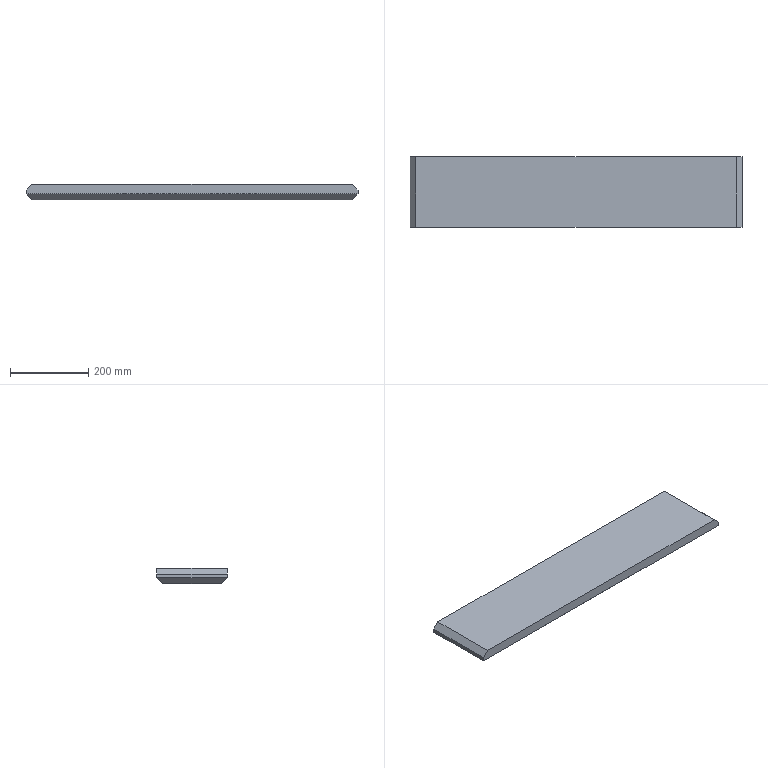Part | SolidWorks | features Chamfer 1, Extrusion 1 | 1 solid | 12 faces | box 850 x 180 x 40 mm | volume 5852250 mm3 | plane 12
STEP:
#1=CARTESIAN_POINT('',(-425.,90.,5.));
#2=VERTEX_POINT('',#1);
#3=CARTESIAN_POINT('',(-425.,90.,-5.));
#4=VERTEX_POINT('',#3);
#5=CARTESIAN_POINT('',(-425.,90.,20.));
#6=DIRECTION('',(0.,0.,-1.));
#7=VECTOR('',#6,1000.);
#8=LINE('',#5,#7);
#9=EDGE_CURVE('',#2,#4,#8,.T.);
#10=ORIENTED_EDGE('',*,*,#9,.T.);
#11=CARTESIAN_POINT('',(-425.,-90.,-5.));
#12=VERTEX_POINT('',#11);
#13=CARTESIAN_POINT('',(-425.,-90.,-5.));
#14=DIRECTION('',(0.,-1.,0.));
#15=VECTOR('',#14,1000.);
#16=LINE('',#13,#15);
#17=EDGE_CURVE('',#4,#12,#16,.T.);
#18=ORIENTED_EDGE('',*,*,#17,.T.);
#19=CARTESIAN_POINT('',(-425.,-90.,5.));
#20=VERTEX_POINT('',#19);
#21=CARTESIAN_POINT('',(-425.,-90.,20.));
#22=DIRECTION('',(0.,0.,-1.));
#23=VECTOR('',#22,1000.);
#24=LINE('',#21,#23);
#25=EDGE_CURVE('',#20,#12,#24,.T.);
#26=ORIENTED_EDGE('',*,*,#25,.F.);
#27=CARTESIAN_POINT('',(-425.,90.,5.));
#28=DIRECTION('',(0.,1.,0.));
#29=VECTOR('',#28,1000.);
#30=LINE('',#27,#29);
#31=EDGE_CURVE('',#20,#2,#30,.T.);
#32=ORIENTED_EDGE('',*,*,#31,.T.);
#33=EDGE_LOOP('',(#10,#18,#26,#32));
#34=FACE_OUTER_BOUND('',#33,.T.);
#35=CARTESIAN_POINT('',(-425.,-90.,20.));
#36=DIRECTION('',(1.,0.,0.));
#37=DIRECTION('',(0.,0.,-1.));
#38=AXIS2_PLACEMENT_3D('',#35,#36,#37);
#39=PLANE('',#38);
#40=ADVANCED_FACE('',(#34),#39,.F.);
#41=ORIENTED_EDGE('',*,*,#25,.T.);
#42=CARTESIAN_POINT('',(425.,-90.,-5.));
#43=VERTEX_POINT('',#42);
#44=CARTESIAN_POINT('',(425.,-90.,-5.));
#45=DIRECTION('',(1.,0.,0.));
#46=VECTOR('',#45,1000.);
#47=LINE('',#44,#46);
#48=EDGE_CURVE('',#12,#43,#47,.T.);
#49=ORIENTED_EDGE('',*,*,#48,.T.);
#50=CARTESIAN_POINT('',(425.,-90.,5.));
#51=VERTEX_POINT('',#50);
#52=CARTESIAN_POINT('',(425.,-90.,20.));
#53=DIRECTION('',(0.,0.,-1.));
#54=VECTOR('',#53,1000.);
#55=LINE('',#52,#54);
#56=EDGE_CURVE('',#51,#43,#55,.T.);
#57=ORIENTED_EDGE('',*,*,#56,.F.);
#58=CARTESIAN_POINT('',(410.,-90.,20.));
#59=VERTEX_POINT('',#58);
#60=CARTESIAN_POINT('',(410.,-90.,20.));
#61=DIRECTION('',(-0.7071,0.,0.7071));
#62=VECTOR('',#61,1000.);
#63=LINE('',#60,#62);
#64=EDGE_CURVE('',#51,#59,#63,.T.);
#65=ORIENTED_EDGE('',*,*,#64,.T.);
#66=CARTESIAN_POINT('',(-410.,-90.,20.));
#67=VERTEX_POINT('',#66);
#68=CARTESIAN_POINT('',(425.,-90.,20.));
#69=DIRECTION('',(1.,0.,0.));
#70=VECTOR('',#69,1000.);
#71=LINE('',#68,#70);
#72=EDGE_CURVE('',#67,#59,#71,.T.);
#73=ORIENTED_EDGE('',*,*,#72,.F.);
#74=CARTESIAN_POINT('',(-410.,-90.,20.));
#75=DIRECTION('',(-0.7071,0.,-0.7071));
#76=VECTOR('',#75,1000.);
#77=LINE('',#74,#76);
#78=EDGE_CURVE('',#67,#20,#77,.T.);
#79=ORIENTED_EDGE('',*,*,#78,.T.);
#80=EDGE_LOOP('',(#41,#49,#57,#65,#73,#79));
#81=FACE_OUTER_BOUND('',#80,.T.);
#82=CARTESIAN_POINT('',(425.,-90.,20.));
#83=DIRECTION('',(0.,1.,0.));
#84=DIRECTION('',(-1.,0.,0.));
#85=AXIS2_PLACEMENT_3D('',#82,#83,#84);
#86=PLANE('',#85);
#87=ADVANCED_FACE('',(#81),#86,.F.);
#88=ORIENTED_EDGE('',*,*,#56,.T.);
#89=CARTESIAN_POINT('',(425.,90.,-5.));
#90=VERTEX_POINT('',#89);
#91=CARTESIAN_POINT('',(425.,-90.,-5.));
#92=DIRECTION('',(0.,1.,0.));
#93=VECTOR('',#92,1000.);
#94=LINE('',#91,#93);
#95=EDGE_CURVE('',#43,#90,#94,.T.);
#96=ORIENTED_EDGE('',*,*,#95,.T.);
#97=CARTESIAN_POINT('',(425.,90.,5.));
#98=VERTEX_POINT('',#97);
#99=CARTESIAN_POINT('',(425.,90.,20.));
#100=DIRECTION('',(0.,0.,-1.));
#101=VECTOR('',#100,1000.);
#102=LINE('',#99,#101);
#103=EDGE_CURVE('',#98,#90,#102,.T.);
#104=ORIENTED_EDGE('',*,*,#103,.F.);
#105=CARTESIAN_POINT('',(425.,-90.,5.));
#106=DIRECTION('',(0.,-1.,0.));
#107=VECTOR('',#106,1000.);
#108=LINE('',#105,#107);
#109=EDGE_CURVE('',#98,#51,#108,.T.);
#110=ORIENTED_EDGE('',*,*,#109,.T.);
#111=EDGE_LOOP('',(#88,#96,#104,#110));
#112=FACE_OUTER_BOUND('',#111,.T.);
#113=CARTESIAN_POINT('',(425.,-90.,20.));
#114=DIRECTION('',(-1.,0.,0.));
#115=DIRECTION('',(0.,0.,1.));
#116=AXIS2_PLACEMENT_3D('',#113,#114,#115);
#117=PLANE('',#116);
#118=ADVANCED_FACE('',(#112),#117,.F.);
#119=ORIENTED_EDGE('',*,*,#103,.T.);
#120=CARTESIAN_POINT('',(425.,90.,-5.));
#121=DIRECTION('',(-1.,0.,0.));
#122=VECTOR('',#121,1000.);
#123=LINE('',#120,#122);
#124=EDGE_CURVE('',#90,#4,#123,.T.);
#125=ORIENTED_EDGE('',*,*,#124,.T.);
#126=ORIENTED_EDGE('',*,*,#9,.F.);
#127=CARTESIAN_POINT('',(-410.,90.,20.));
#128=VERTEX_POINT('',#127);
#129=CARTESIAN_POINT('',(-410.,90.,20.));
#130=DIRECTION('',(0.7071,0.,0.7071));
#131=VECTOR('',#130,1000.);
#132=LINE('',#129,#131);
#133=EDGE_CURVE('',#2,#128,#132,.T.);
#134=ORIENTED_EDGE('',*,*,#133,.T.);
#135=CARTESIAN_POINT('',(410.,90.,20.));
#136=VERTEX_POINT('',#135);
#137=CARTESIAN_POINT('',(425.,90.,20.));
#138=DIRECTION('',(-1.,0.,0.));
#139=VECTOR('',#138,1000.);
#140=LINE('',#137,#139);
#141=EDGE_CURVE('',#136,#128,#140,.T.);
#142=ORIENTED_EDGE('',*,*,#141,.F.);
#143=CARTESIAN_POINT('',(410.,90.,20.));
#144=DIRECTION('',(0.7071,0.,-0.7071));
#145=VECTOR('',#144,1000.);
#146=LINE('',#143,#145);
#147=EDGE_CURVE('',#136,#98,#146,.T.);
#148=ORIENTED_EDGE('',*,*,#147,.T.);
#149=EDGE_LOOP('',(#119,#125,#126,#134,#142,#148));
#150=FACE_OUTER_BOUND('',#149,.T.);
#151=CARTESIAN_POINT('',(425.,90.,20.));
#152=DIRECTION('',(0.,-1.,0.));
#153=DIRECTION('',(1.,0.,0.));
#154=AXIS2_PLACEMENT_3D('',#151,#152,#153);
#155=PLANE('',#154);
#156=ADVANCED_FACE('',(#150),#155,.F.);
#157=ORIENTED_EDGE('',*,*,#72,.T.);
#158=CARTESIAN_POINT('',(410.,90.,20.));
#159=DIRECTION('',(0.,1.,0.));
#160=VECTOR('',#159,1000.);
#161=LINE('',#158,#160);
#162=EDGE_CURVE('',#59,#136,#161,.T.);
#163=ORIENTED_EDGE('',*,*,#162,.T.);
#164=ORIENTED_EDGE('',*,*,#141,.T.);
#165=CARTESIAN_POINT('',(-410.,-90.,20.));
#166=DIRECTION('',(0.,-1.,0.));
#167=VECTOR('',#166,1000.);
#168=LINE('',#165,#167);
#169=EDGE_CURVE('',#128,#67,#168,.T.);
#170=ORIENTED_EDGE('',*,*,#169,.T.);
#171=EDGE_LOOP('',(#157,#163,#164,#170));
#172=FACE_OUTER_BOUND('',#171,.T.);
#173=CARTESIAN_POINT('',(0.,0.,20.));
#174=DIRECTION('',(0.,0.,1.));
#175=DIRECTION('',(1.,0.,0.));
#176=AXIS2_PLACEMENT_3D('',#173,#174,#175);
#177=PLANE('',#176);
#178=ADVANCED_FACE('',(#172),#177,.T.);
#179=CARTESIAN_POINT('',(410.,75.,-20.));
#180=VERTEX_POINT('',#179);
#181=CARTESIAN_POINT('',(410.,-75.,-20.));
#182=VERTEX_POINT('',#181);
#183=CARTESIAN_POINT('',(410.,0.,-20.));
#184=DIRECTION('',(0.,-1.,0.));
#185=VECTOR('',#184,1000.);
#186=LINE('',#183,#185);
#187=EDGE_CURVE('',#180,#182,#186,.T.);
#188=ORIENTED_EDGE('',*,*,#187,.T.);
#189=CARTESIAN_POINT('',(-410.,-75.,-20.));
#190=VERTEX_POINT('',#189);
#191=CARTESIAN_POINT('',(0.,-75.,-20.));
#192=DIRECTION('',(-1.,0.,0.));
#193=VECTOR('',#192,1000.);
#194=LINE('',#191,#193);
#195=EDGE_CURVE('',#182,#190,#194,.T.);
#196=ORIENTED_EDGE('',*,*,#195,.T.);
#197=CARTESIAN_POINT('',(-410.,75.,-20.));
#198=VERTEX_POINT('',#197);
#199=CARTESIAN_POINT('',(-410.,0.,-20.));
#200=DIRECTION('',(0.,1.,0.));
#201=VECTOR('',#200,1000.);
#202=LINE('',#199,#201);
#203=EDGE_CURVE('',#190,#198,#202,.T.);
#204=ORIENTED_EDGE('',*,*,#203,.T.);
#205=CARTESIAN_POINT('',(0.,75.,-20.));
#206=DIRECTION('',(1.,0.,0.));
#207=VECTOR('',#206,1000.);
#208=LINE('',#205,#207);
#209=EDGE_CURVE('',#198,#180,#208,.T.);
#210=ORIENTED_EDGE('',*,*,#209,.T.);
#211=EDGE_LOOP('',(#188,#196,#204,#210));
#212=FACE_OUTER_BOUND('',#211,.T.);
#213=CARTESIAN_POINT('',(0.,0.,-20.));
#214=DIRECTION('',(0.,0.,1.));
#215=DIRECTION('',(1.,0.,0.));
#216=AXIS2_PLACEMENT_3D('',#213,#214,#215);
#217=PLANE('',#216);
#218=ADVANCED_FACE('',(#212),#217,.F.);
#219=CARTESIAN_POINT('',(425.,90.,-5.));
#220=DIRECTION('',(0.5774,0.5774,0.5774));
#221=VECTOR('',#220,1000.);
#222=LINE('',#219,#221);
#223=EDGE_CURVE('',#180,#90,#222,.T.);
#224=ORIENTED_EDGE('',*,*,#223,.F.);
#225=ORIENTED_EDGE('',*,*,#209,.F.);
#226=CARTESIAN_POINT('',(-365.,30.,-65.));
#227=DIRECTION('',(0.5774,-0.5774,-0.5774));
#228=VECTOR('',#227,1000.);
#229=LINE('',#226,#228);
#230=EDGE_CURVE('',#4,#198,#229,.T.);
#231=ORIENTED_EDGE('',*,*,#230,.F.);
#232=ORIENTED_EDGE('',*,*,#124,.F.);
#233=EDGE_LOOP('',(#224,#225,#231,#232));
#234=FACE_OUTER_BOUND('',#233,.T.);
#235=CARTESIAN_POINT('',(425.,90.,-5.));
#236=DIRECTION('',(0.,-0.7071,0.7071));
#237=DIRECTION('',(-1.,0.,0.));
#238=AXIS2_PLACEMENT_3D('',#235,#236,#237);
#239=PLANE('',#238);
#240=ADVANCED_FACE('',(#234),#239,.F.);
#241=ORIENTED_EDGE('',*,*,#230,.T.);
#242=ORIENTED_EDGE('',*,*,#203,.F.);
#243=CARTESIAN_POINT('',(-425.,-90.,-5.));
#244=DIRECTION('',(0.5774,0.5774,-0.5774));
#245=VECTOR('',#244,1000.);
#246=LINE('',#243,#245);
#247=EDGE_CURVE('',#12,#190,#246,.T.);
#248=ORIENTED_EDGE('',*,*,#247,.F.);
#249=ORIENTED_EDGE('',*,*,#17,.F.);
#250=EDGE_LOOP('',(#241,#242,#248,#249));
#251=FACE_OUTER_BOUND('',#250,.T.);
#252=CARTESIAN_POINT('',(-425.,-90.,-5.));
#253=DIRECTION('',(0.7071,0.,0.7071));
#254=DIRECTION('',(0.,-1.,0.));
#255=AXIS2_PLACEMENT_3D('',#252,#253,#254);
#256=PLANE('',#255);
#257=ADVANCED_FACE('',(#251),#256,.F.);
#258=ORIENTED_EDGE('',*,*,#223,.T.);
#259=ORIENTED_EDGE('',*,*,#95,.F.);
#260=CARTESIAN_POINT('',(425.,-90.,-5.));
#261=DIRECTION('',(0.5774,-0.5774,0.5774));
#262=VECTOR('',#261,1000.);
#263=LINE('',#260,#262);
#264=EDGE_CURVE('',#182,#43,#263,.T.);
#265=ORIENTED_EDGE('',*,*,#264,.F.);
#266=ORIENTED_EDGE('',*,*,#187,.F.);
#267=EDGE_LOOP('',(#258,#259,#265,#266));
#268=FACE_OUTER_BOUND('',#267,.T.);
#269=CARTESIAN_POINT('',(425.,-90.,-5.));
#270=DIRECTION('',(-0.7071,0.,0.7071));
#271=DIRECTION('',(0.,1.,0.));
#272=AXIS2_PLACEMENT_3D('',#269,#270,#271);
#273=PLANE('',#272);
#274=ADVANCED_FACE('',(#268),#273,.F.);
#275=ORIENTED_EDGE('',*,*,#247,.T.);
#276=ORIENTED_EDGE('',*,*,#195,.F.);
#277=ORIENTED_EDGE('',*,*,#264,.T.);
#278=ORIENTED_EDGE('',*,*,#48,.F.);
#279=EDGE_LOOP('',(#275,#276,#277,#278));
#280=FACE_OUTER_BOUND('',#279,.T.);
#281=CARTESIAN_POINT('',(425.,-90.,-5.));
#282=DIRECTION('',(0.,0.7071,0.7071));
#283=DIRECTION('',(1.,0.,0.));
#284=AXIS2_PLACEMENT_3D('',#281,#282,#283);
#285=PLANE('',#284);
#286=ADVANCED_FACE('',(#280),#285,.F.);
#287=ORIENTED_EDGE('',*,*,#64,.F.);
#288=ORIENTED_EDGE('',*,*,#109,.F.);
#289=ORIENTED_EDGE('',*,*,#147,.F.);
#290=ORIENTED_EDGE('',*,*,#162,.F.);
#291=EDGE_LOOP('',(#287,#288,#289,#290));
#292=FACE_OUTER_BOUND('',#291,.T.);
#293=CARTESIAN_POINT('',(410.,0.,20.));
#294=DIRECTION('',(0.7071,0.,0.7071));
#295=DIRECTION('',(0.,-1.,0.));
#296=AXIS2_PLACEMENT_3D('',#293,#294,#295);
#297=PLANE('',#296);
#298=ADVANCED_FACE('',(#292),#297,.T.);
#299=ORIENTED_EDGE('',*,*,#133,.F.);
#300=ORIENTED_EDGE('',*,*,#31,.F.);
#301=ORIENTED_EDGE('',*,*,#78,.F.);
#302=ORIENTED_EDGE('',*,*,#169,.F.);
#303=EDGE_LOOP('',(#299,#300,#301,#302));
#304=FACE_OUTER_BOUND('',#303,.T.);
#305=CARTESIAN_POINT('',(-410.,0.,20.));
#306=DIRECTION('',(-0.7071,0.,0.7071));
#307=DIRECTION('',(0.,1.,0.));
#308=AXIS2_PLACEMENT_3D('',#305,#306,#307);
#309=PLANE('',#308);
#310=ADVANCED_FACE('',(#304),#309,.T.);
#311=CLOSED_SHELL('',(#40,#87,#118,#156,#178,#218,#240,#257,#274,#286,#298,#310));
#312=MANIFOLD_SOLID_BREP('',#311);
#313=CARTESIAN_POINT('',(0.,0.,0.));
#314=DIRECTION('',(0.,0.,1.));
#315=DIRECTION('',(1.,0.,0.));
#316=AXIS2_PLACEMENT_3D('',#313,#314,#315);
#317=(LENGTH_UNIT()NAMED_UNIT(*)SI_UNIT(.MILLI.,.METRE.));
#318=UNCERTAINTY_MEASURE_WITH_UNIT(LENGTH_MEASURE(0.00001),#317,'','');
#319=(NAMED_UNIT(*)PLANE_ANGLE_UNIT()SI_UNIT($,.RADIAN.));
#320=(NAMED_UNIT(*)SI_UNIT($,.STERADIAN.)SOLID_ANGLE_UNIT());
#321=(GEOMETRIC_REPRESENTATION_CONTEXT(3)GLOBAL_UNCERTAINTY_ASSIGNED_CONTEXT((#318))GLOBAL_UNIT_ASSIGNED_CONTEXT((#317,#319,#320))REPRESENTATION_CONTEXT('',''));
#322=ADVANCED_BREP_SHAPE_REPRESENTATION('',(#312,#316),#321);